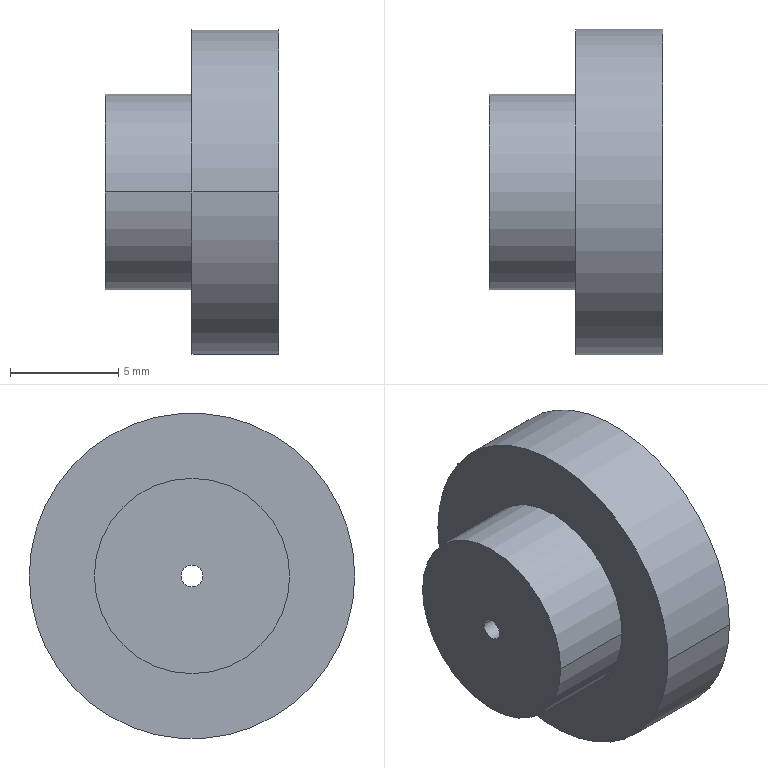Part | SolidWorks | features Revolution 1 | 1 solid | 11 faces | box 8 x 15 x 15 mm | volume 928.864 mm3 | cylinder 6 | plane 3 | cone 2 | commonest cylinder face diameters 1 x2 9 x2 15 x2
STEP:
#1=CARTESIAN_POINT('',(0.,4.5,0.));
#2=VERTEX_POINT('',#1);
#3=CARTESIAN_POINT('',(0.,-4.5,0.));
#4=VERTEX_POINT('',#3);
#5=CARTESIAN_POINT('',(0.,0.,0.));
#6=DIRECTION('',(1.,0.,0.));
#7=DIRECTION('',(0.,1.,0.));
#8=AXIS2_PLACEMENT_3D('',#5,#6,#7);
#9=CIRCLE('',#8,4.5);
#10=EDGE_CURVE('',#2,#4,#9,.T.);
#11=ORIENTED_EDGE('',*,*,#10,.T.);
#12=CARTESIAN_POINT('',(4.,-4.5,0.));
#13=VERTEX_POINT('',#12);
#14=CARTESIAN_POINT('',(8.,-4.5,0.));
#15=DIRECTION('',(1.,0.,0.));
#16=VECTOR('',#15,1000.);
#17=LINE('',#14,#16);
#18=EDGE_CURVE('',#4,#13,#17,.T.);
#19=ORIENTED_EDGE('',*,*,#18,.T.);
#20=CARTESIAN_POINT('',(4.,4.5,0.));
#21=VERTEX_POINT('',#20);
#22=CARTESIAN_POINT('',(4.,0.,0.));
#23=DIRECTION('',(1.,0.,0.));
#24=DIRECTION('',(0.,1.,0.));
#25=AXIS2_PLACEMENT_3D('',#22,#23,#24);
#26=CIRCLE('',#25,4.5);
#27=EDGE_CURVE('',#21,#13,#26,.T.);
#28=ORIENTED_EDGE('',*,*,#27,.F.);
#29=CARTESIAN_POINT('',(8.,4.5,0.));
#30=DIRECTION('',(1.,0.,0.));
#31=VECTOR('',#30,1000.);
#32=LINE('',#29,#31);
#33=EDGE_CURVE('',#2,#21,#32,.T.);
#34=ORIENTED_EDGE('',*,*,#33,.F.);
#35=EDGE_LOOP('',(#11,#19,#28,#34));
#36=FACE_OUTER_BOUND('',#35,.T.);
#37=CARTESIAN_POINT('',(8.,0.,0.));
#38=DIRECTION('',(1.,0.,0.));
#39=DIRECTION('',(0.,1.,0.));
#40=AXIS2_PLACEMENT_3D('',#37,#38,#39);
#41=CYLINDRICAL_SURFACE('',#40,4.5);
#42=ADVANCED_FACE('',(#36),#41,.T.);
#43=CARTESIAN_POINT('',(4.,7.5,0.));
#44=VERTEX_POINT('',#43);
#45=CARTESIAN_POINT('',(4.,-7.5,0.));
#46=VERTEX_POINT('',#45);
#47=CARTESIAN_POINT('',(4.,0.,0.));
#48=DIRECTION('',(1.,0.,0.));
#49=DIRECTION('',(0.,1.,0.));
#50=AXIS2_PLACEMENT_3D('',#47,#48,#49);
#51=CIRCLE('',#50,7.5);
#52=EDGE_CURVE('',#44,#46,#51,.T.);
#53=ORIENTED_EDGE('',*,*,#52,.T.);
#54=CARTESIAN_POINT('',(8.,-7.5,0.));
#55=VERTEX_POINT('',#54);
#56=CARTESIAN_POINT('',(8.,-7.5,0.));
#57=DIRECTION('',(1.,0.,0.));
#58=VECTOR('',#57,1000.);
#59=LINE('',#56,#58);
#60=EDGE_CURVE('',#46,#55,#59,.T.);
#61=ORIENTED_EDGE('',*,*,#60,.T.);
#62=CARTESIAN_POINT('',(8.,7.5,0.));
#63=VERTEX_POINT('',#62);
#64=CARTESIAN_POINT('',(8.,0.,0.));
#65=DIRECTION('',(1.,0.,0.));
#66=DIRECTION('',(0.,1.,0.));
#67=AXIS2_PLACEMENT_3D('',#64,#65,#66);
#68=CIRCLE('',#67,7.5);
#69=EDGE_CURVE('',#63,#55,#68,.T.);
#70=ORIENTED_EDGE('',*,*,#69,.F.);
#71=CARTESIAN_POINT('',(8.,7.5,0.));
#72=DIRECTION('',(1.,0.,0.));
#73=VECTOR('',#72,1000.);
#74=LINE('',#71,#73);
#75=EDGE_CURVE('',#44,#63,#74,.T.);
#76=ORIENTED_EDGE('',*,*,#75,.F.);
#77=EDGE_LOOP('',(#53,#61,#70,#76));
#78=FACE_OUTER_BOUND('',#77,.T.);
#79=CARTESIAN_POINT('',(8.,0.,0.));
#80=DIRECTION('',(1.,0.,0.));
#81=DIRECTION('',(0.,1.,0.));
#82=AXIS2_PLACEMENT_3D('',#79,#80,#81);
#83=CYLINDRICAL_SURFACE('',#82,7.5);
#84=ADVANCED_FACE('',(#78),#83,.T.);
#85=CARTESIAN_POINT('',(5.5,-0.5,0.));
#86=VERTEX_POINT('',#85);
#87=CARTESIAN_POINT('',(5.5,0.5,0.));
#88=VERTEX_POINT('',#87);
#89=CARTESIAN_POINT('',(5.5,0.,0.));
#90=DIRECTION('',(1.,0.,0.));
#91=DIRECTION('',(0.,1.,0.));
#92=AXIS2_PLACEMENT_3D('',#89,#90,#91);
#93=CIRCLE('',#92,0.5);
#94=EDGE_CURVE('',#86,#88,#93,.T.);
#95=ORIENTED_EDGE('',*,*,#94,.F.);
#96=CARTESIAN_POINT('',(8.,-3.,0.));
#97=VERTEX_POINT('',#96);
#98=CARTESIAN_POINT('',(5.5,-0.5,0.));
#99=DIRECTION('',(0.7071,-0.7071,0.));
#100=VECTOR('',#99,1000.);
#101=LINE('',#98,#100);
#102=EDGE_CURVE('',#86,#97,#101,.T.);
#103=ORIENTED_EDGE('',*,*,#102,.T.);
#104=CARTESIAN_POINT('',(8.,3.,0.));
#105=VERTEX_POINT('',#104);
#106=CARTESIAN_POINT('',(8.,0.,0.));
#107=DIRECTION('',(1.,0.,0.));
#108=DIRECTION('',(0.,1.,0.));
#109=AXIS2_PLACEMENT_3D('',#106,#107,#108);
#110=CIRCLE('',#109,3.);
#111=EDGE_CURVE('',#97,#105,#110,.T.);
#112=ORIENTED_EDGE('',*,*,#111,.T.);
#113=CARTESIAN_POINT('',(5.5,0.5,0.));
#114=DIRECTION('',(0.7071,0.7071,0.));
#115=VECTOR('',#114,1000.);
#116=LINE('',#113,#115);
#117=EDGE_CURVE('',#88,#105,#116,.T.);
#118=ORIENTED_EDGE('',*,*,#117,.F.);
#119=EDGE_LOOP('',(#95,#103,#112,#118));
#120=FACE_OUTER_BOUND('',#119,.T.);
#121=CARTESIAN_POINT('',(5.5,0.,0.));
#122=DIRECTION('',(1.,0.,0.));
#123=DIRECTION('',(0.,1.,0.));
#124=AXIS2_PLACEMENT_3D('',#121,#122,#123);
#125=CONICAL_SURFACE('',#124,0.5,0.7854);
#126=ADVANCED_FACE('',(#120),#125,.F.);
#127=CARTESIAN_POINT('',(0.,-0.5,0.));
#128=VERTEX_POINT('',#127);
#129=CARTESIAN_POINT('',(0.,0.5,0.));
#130=VERTEX_POINT('',#129);
#131=CARTESIAN_POINT('',(0.,0.,0.));
#132=DIRECTION('',(1.,0.,0.));
#133=DIRECTION('',(0.,1.,0.));
#134=AXIS2_PLACEMENT_3D('',#131,#132,#133);
#135=CIRCLE('',#134,0.5);
#136=EDGE_CURVE('',#128,#130,#135,.T.);
#137=ORIENTED_EDGE('',*,*,#136,.F.);
#138=CARTESIAN_POINT('',(8.,-0.5,0.));
#139=DIRECTION('',(1.,0.,0.));
#140=VECTOR('',#139,1000.);
#141=LINE('',#138,#140);
#142=EDGE_CURVE('',#128,#86,#141,.T.);
#143=ORIENTED_EDGE('',*,*,#142,.T.);
#144=ORIENTED_EDGE('',*,*,#94,.T.);
#145=CARTESIAN_POINT('',(8.,0.5,0.));
#146=DIRECTION('',(1.,0.,0.));
#147=VECTOR('',#146,1000.);
#148=LINE('',#145,#147);
#149=EDGE_CURVE('',#130,#88,#148,.T.);
#150=ORIENTED_EDGE('',*,*,#149,.F.);
#151=EDGE_LOOP('',(#137,#143,#144,#150));
#152=FACE_OUTER_BOUND('',#151,.T.);
#153=CARTESIAN_POINT('',(8.,0.,0.));
#154=DIRECTION('',(1.,0.,0.));
#155=DIRECTION('',(0.,1.,0.));
#156=AXIS2_PLACEMENT_3D('',#153,#154,#155);
#157=CYLINDRICAL_SURFACE('',#156,0.5);
#158=ADVANCED_FACE('',(#152),#157,.F.);
#159=ORIENTED_EDGE('',*,*,#142,.F.);
#160=CARTESIAN_POINT('',(0.,0.,0.));
#161=DIRECTION('',(1.,0.,0.));
#162=DIRECTION('',(0.,1.,0.));
#163=AXIS2_PLACEMENT_3D('',#160,#161,#162);
#164=CIRCLE('',#163,0.5);
#165=EDGE_CURVE('',#130,#128,#164,.T.);
#166=ORIENTED_EDGE('',*,*,#165,.F.);
#167=ORIENTED_EDGE('',*,*,#149,.T.);
#168=CARTESIAN_POINT('',(5.5,0.,0.));
#169=DIRECTION('',(1.,0.,0.));
#170=DIRECTION('',(0.,1.,0.));
#171=AXIS2_PLACEMENT_3D('',#168,#169,#170);
#172=CIRCLE('',#171,0.5);
#173=EDGE_CURVE('',#88,#86,#172,.T.);
#174=ORIENTED_EDGE('',*,*,#173,.T.);
#175=EDGE_LOOP('',(#159,#166,#167,#174));
#176=FACE_OUTER_BOUND('',#175,.T.);
#177=CARTESIAN_POINT('',(8.,0.,0.));
#178=DIRECTION('',(1.,0.,0.));
#179=DIRECTION('',(0.,1.,0.));
#180=AXIS2_PLACEMENT_3D('',#177,#178,#179);
#181=CYLINDRICAL_SURFACE('',#180,0.5);
#182=ADVANCED_FACE('',(#176),#181,.F.);
#183=ORIENTED_EDGE('',*,*,#102,.F.);
#184=ORIENTED_EDGE('',*,*,#173,.F.);
#185=ORIENTED_EDGE('',*,*,#117,.T.);
#186=CARTESIAN_POINT('',(8.,0.,0.));
#187=DIRECTION('',(1.,0.,0.));
#188=DIRECTION('',(0.,1.,0.));
#189=AXIS2_PLACEMENT_3D('',#186,#187,#188);
#190=CIRCLE('',#189,3.);
#191=EDGE_CURVE('',#105,#97,#190,.T.);
#192=ORIENTED_EDGE('',*,*,#191,.T.);
#193=EDGE_LOOP('',(#183,#184,#185,#192));
#194=FACE_OUTER_BOUND('',#193,.T.);
#195=CARTESIAN_POINT('',(5.5,0.,0.));
#196=DIRECTION('',(1.,0.,0.));
#197=DIRECTION('',(0.,1.,0.));
#198=AXIS2_PLACEMENT_3D('',#195,#196,#197);
#199=CONICAL_SURFACE('',#198,0.5,0.7854);
#200=ADVANCED_FACE('',(#194),#199,.F.);
#201=ORIENTED_EDGE('',*,*,#191,.F.);
#202=ORIENTED_EDGE('',*,*,#111,.F.);
#203=EDGE_LOOP('',(#201,#202));
#204=FACE_BOUND('',#203,.T.);
#205=ORIENTED_EDGE('',*,*,#69,.T.);
#206=CARTESIAN_POINT('',(8.,0.,0.));
#207=DIRECTION('',(1.,0.,0.));
#208=DIRECTION('',(0.,1.,0.));
#209=AXIS2_PLACEMENT_3D('',#206,#207,#208);
#210=CIRCLE('',#209,7.5);
#211=EDGE_CURVE('',#55,#63,#210,.T.);
#212=ORIENTED_EDGE('',*,*,#211,.T.);
#213=EDGE_LOOP('',(#205,#212));
#214=FACE_OUTER_BOUND('',#213,.T.);
#215=CARTESIAN_POINT('',(8.,0.,0.));
#216=DIRECTION('',(-1.,0.,0.));
#217=DIRECTION('',(0.,-1.,0.));
#218=AXIS2_PLACEMENT_3D('',#215,#216,#217);
#219=PLANE('',#218);
#220=ADVANCED_FACE('',(#204,#214),#219,.F.);
#221=ORIENTED_EDGE('',*,*,#60,.F.);
#222=CARTESIAN_POINT('',(4.,0.,0.));
#223=DIRECTION('',(1.,0.,0.));
#224=DIRECTION('',(0.,1.,0.));
#225=AXIS2_PLACEMENT_3D('',#222,#223,#224);
#226=CIRCLE('',#225,7.5);
#227=EDGE_CURVE('',#46,#44,#226,.T.);
#228=ORIENTED_EDGE('',*,*,#227,.T.);
#229=ORIENTED_EDGE('',*,*,#75,.T.);
#230=ORIENTED_EDGE('',*,*,#211,.F.);
#231=EDGE_LOOP('',(#221,#228,#229,#230));
#232=FACE_OUTER_BOUND('',#231,.T.);
#233=CARTESIAN_POINT('',(8.,0.,0.));
#234=DIRECTION('',(1.,0.,0.));
#235=DIRECTION('',(0.,1.,0.));
#236=AXIS2_PLACEMENT_3D('',#233,#234,#235);
#237=CYLINDRICAL_SURFACE('',#236,7.5);
#238=ADVANCED_FACE('',(#232),#237,.T.);
#239=ORIENTED_EDGE('',*,*,#52,.F.);
#240=ORIENTED_EDGE('',*,*,#227,.F.);
#241=EDGE_LOOP('',(#239,#240));
#242=FACE_OUTER_BOUND('',#241,.T.);
#243=ORIENTED_EDGE('',*,*,#27,.T.);
#244=CARTESIAN_POINT('',(4.,0.,0.));
#245=DIRECTION('',(1.,0.,0.));
#246=DIRECTION('',(0.,1.,0.));
#247=AXIS2_PLACEMENT_3D('',#244,#245,#246);
#248=CIRCLE('',#247,4.5);
#249=EDGE_CURVE('',#13,#21,#248,.T.);
#250=ORIENTED_EDGE('',*,*,#249,.T.);
#251=EDGE_LOOP('',(#243,#250));
#252=FACE_BOUND('',#251,.T.);
#253=CARTESIAN_POINT('',(4.,0.,0.));
#254=DIRECTION('',(1.,0.,0.));
#255=DIRECTION('',(0.,1.,0.));
#256=AXIS2_PLACEMENT_3D('',#253,#254,#255);
#257=PLANE('',#256);
#258=ADVANCED_FACE('',(#242,#252),#257,.F.);
#259=ORIENTED_EDGE('',*,*,#18,.F.);
#260=CARTESIAN_POINT('',(0.,0.,0.));
#261=DIRECTION('',(1.,0.,0.));
#262=DIRECTION('',(0.,1.,0.));
#263=AXIS2_PLACEMENT_3D('',#260,#261,#262);
#264=CIRCLE('',#263,4.5);
#265=EDGE_CURVE('',#4,#2,#264,.T.);
#266=ORIENTED_EDGE('',*,*,#265,.T.);
#267=ORIENTED_EDGE('',*,*,#33,.T.);
#268=ORIENTED_EDGE('',*,*,#249,.F.);
#269=EDGE_LOOP('',(#259,#266,#267,#268));
#270=FACE_OUTER_BOUND('',#269,.T.);
#271=CARTESIAN_POINT('',(8.,0.,0.));
#272=DIRECTION('',(1.,0.,0.));
#273=DIRECTION('',(0.,1.,0.));
#274=AXIS2_PLACEMENT_3D('',#271,#272,#273);
#275=CYLINDRICAL_SURFACE('',#274,4.5);
#276=ADVANCED_FACE('',(#270),#275,.T.);
#277=ORIENTED_EDGE('',*,*,#10,.F.);
#278=ORIENTED_EDGE('',*,*,#265,.F.);
#279=EDGE_LOOP('',(#277,#278));
#280=FACE_OUTER_BOUND('',#279,.T.);
#281=ORIENTED_EDGE('',*,*,#165,.T.);
#282=ORIENTED_EDGE('',*,*,#136,.T.);
#283=EDGE_LOOP('',(#281,#282));
#284=FACE_BOUND('',#283,.T.);
#285=CARTESIAN_POINT('',(0.,0.,0.));
#286=DIRECTION('',(1.,0.,0.));
#287=DIRECTION('',(0.,1.,0.));
#288=AXIS2_PLACEMENT_3D('',#285,#286,#287);
#289=PLANE('',#288);
#290=ADVANCED_FACE('',(#280,#284),#289,.F.);
#291=CLOSED_SHELL('',(#42,#84,#126,#158,#182,#200,#220,#238,#258,#276,#290));
#292=MANIFOLD_SOLID_BREP('',#291);
#293=CARTESIAN_POINT('',(0.,0.,0.));
#294=DIRECTION('',(0.,0.,1.));
#295=DIRECTION('',(1.,0.,0.));
#296=AXIS2_PLACEMENT_3D('',#293,#294,#295);
#297=(LENGTH_UNIT()NAMED_UNIT(*)SI_UNIT(.MILLI.,.METRE.));
#298=UNCERTAINTY_MEASURE_WITH_UNIT(LENGTH_MEASURE(0.00001),#297,'','');
#299=(NAMED_UNIT(*)PLANE_ANGLE_UNIT()SI_UNIT($,.RADIAN.));
#300=(NAMED_UNIT(*)SI_UNIT($,.STERADIAN.)SOLID_ANGLE_UNIT());
#301=(GEOMETRIC_REPRESENTATION_CONTEXT(3)GLOBAL_UNCERTAINTY_ASSIGNED_CONTEXT((#298))GLOBAL_UNIT_ASSIGNED_CONTEXT((#297,#299,#300))REPRESENTATION_CONTEXT('',''));
#302=ADVANCED_BREP_SHAPE_REPRESENTATION('',(#292,#296),#301);